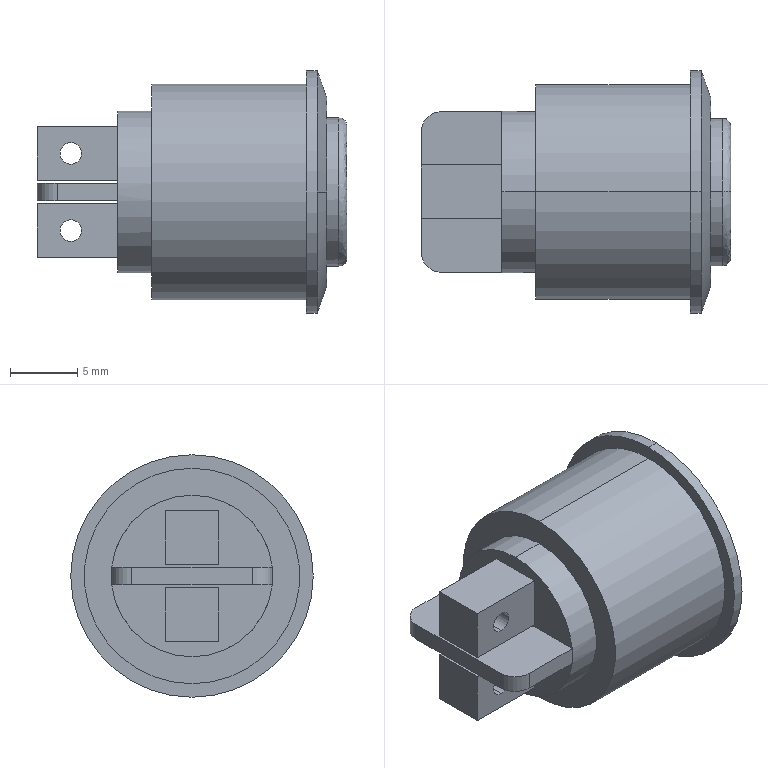Part | SolidWorks | features BaseBody 1 | 1 solid | 41 faces | box 23 x 18 x 18 mm | volume 3351 mm3 | plane 23 | cylinder 14 | spline 2 | cone 2 | commonest cylinder face diameters 1.6 x4 3 x2 11 x2 12 x2 16 x2 18 x2
STEP:
#1=CARTESIAN_POINT('',(3.,0.,4.9));
#2=VERTEX_POINT('',#1);
#3=CARTESIAN_POINT('',(3.,0.04193,4.9));
#4=VERTEX_POINT('',#3);
#5=CARTESIAN_POINT('',(3.,0.,4.9));
#6=CARTESIAN_POINT('',(3.,0.01398,4.9));
#7=CARTESIAN_POINT('',(3.,0.02796,4.9));
#8=CARTESIAN_POINT('',(3.,0.04193,4.9));
#9=(BOUNDED_CURVE()B_SPLINE_CURVE(3,(#5,#6,#7,#8),.UNSPECIFIED.,.F.,.F.)B_SPLINE_CURVE_WITH_KNOTS((4,4),(0.,0.002724),.UNSPECIFIED.)CURVE()GEOMETRIC_REPRESENTATION_ITEM()RATIONAL_B_SPLINE_CURVE((1.,1.,1.,1.))REPRESENTATION_ITEM(''));
#10=EDGE_CURVE('',#2,#4,#9,.T.);
#11=ORIENTED_EDGE('',*,*,#10,.T.);
#12=CARTESIAN_POINT('',(2.4,0.04707,5.5));
#13=VERTEX_POINT('',#12);
#14=CARTESIAN_POINT('',(2.4,0.04193,4.9));
#15=DIRECTION('',(0.,-1.,0.008558));
#16=DIRECTION('',(0.,0.008558,1.));
#17=AXIS2_PLACEMENT_3D('',#14,#15,#16);
#18=CIRCLE('',#17,0.6);
#19=EDGE_CURVE('',#4,#13,#18,.T.);
#20=ORIENTED_EDGE('',*,*,#19,.T.);
#21=CARTESIAN_POINT('',(2.4,0.,5.5));
#22=VERTEX_POINT('',#21);
#23=CARTESIAN_POINT('',(2.4,0.,0.));
#24=DIRECTION('',(-1.,0.,0.));
#25=DIRECTION('',(0.,0.,-1.));
#26=AXIS2_PLACEMENT_3D('',#23,#24,#25);
#27=CIRCLE('',#26,5.5);
#28=EDGE_CURVE('',#22,#13,#27,.T.);
#29=ORIENTED_EDGE('',*,*,#28,.F.);
#30=CARTESIAN_POINT('',(2.4,-0.04707,-5.5));
#31=VERTEX_POINT('',#30);
#32=CARTESIAN_POINT('',(2.4,0.,0.));
#33=DIRECTION('',(-1.,0.,0.));
#34=DIRECTION('',(0.,0.,-1.));
#35=AXIS2_PLACEMENT_3D('',#32,#33,#34);
#36=CIRCLE('',#35,5.5);
#37=EDGE_CURVE('',#31,#22,#36,.T.);
#38=ORIENTED_EDGE('',*,*,#37,.F.);
#39=CARTESIAN_POINT('',(3.,-0.04193,-4.9));
#40=VERTEX_POINT('',#39);
#41=CARTESIAN_POINT('',(2.4,-0.04193,-4.9));
#42=DIRECTION('',(0.,1.,-0.008558));
#43=DIRECTION('',(0.,-0.008558,-1.));
#44=AXIS2_PLACEMENT_3D('',#41,#42,#43);
#45=CIRCLE('',#44,0.6);
#46=EDGE_CURVE('',#40,#31,#45,.T.);
#47=ORIENTED_EDGE('',*,*,#46,.F.);
#48=CARTESIAN_POINT('',(3.,-0.04193,-4.9));
#49=CARTESIAN_POINT('',(3.,-0.1202,-4.899));
#50=CARTESIAN_POINT('',(3.,-0.2018,-4.897));
#51=CARTESIAN_POINT('',(3.,-0.3615,-4.887));
#52=CARTESIAN_POINT('',(3.,-0.4412,-4.881));
#53=CARTESIAN_POINT('',(3.,-0.6798,-4.855));
#54=CARTESIAN_POINT('',(3.,-0.838,-4.831));
#55=CARTESIAN_POINT('',(3.,-1.308,-4.733));
#56=CARTESIAN_POINT('',(3.,-1.615,-4.637));
#57=CARTESIAN_POINT('',(3.,-2.498,-4.264));
#58=CARTESIAN_POINT('',(3.,-3.038,-3.898));
#59=CARTESIAN_POINT('',(3.,-3.937,-2.987));
#60=CARTESIAN_POINT('',(3.,-4.296,-2.443));
#61=CARTESIAN_POINT('',(3.,-4.779,-1.258));
#62=CARTESIAN_POINT('',(3.,-4.903,-0.6179));
#63=CARTESIAN_POINT('',(3.,-4.9,0.02429));
#64=CARTESIAN_POINT('',(3.,-4.9,0.02398));
#65=CARTESIAN_POINT('',(3.,-4.9,0.02623));
#66=CARTESIAN_POINT('',(3.,-4.9,0.02966));
#67=CARTESIAN_POINT('',(3.,-4.9,0.03811));
#68=CARTESIAN_POINT('',(3.,-4.9,0.05674));
#69=CARTESIAN_POINT('',(3.,-4.899,0.07569));
#70=CARTESIAN_POINT('',(3.,-4.899,0.1176));
#71=CARTESIAN_POINT('',(3.,-4.898,0.1508));
#72=CARTESIAN_POINT('',(3.,-4.894,0.2663));
#73=CARTESIAN_POINT('',(3.,-4.888,0.3645));
#74=CARTESIAN_POINT('',(3.,-4.876,0.4909));
#75=CARTESIAN_POINT('',(3.,-4.875,0.4945));
#76=CARTESIAN_POINT('',(3.,-4.874,0.5055));
#77=CARTESIAN_POINT('',(3.,-4.873,0.5219));
#78=CARTESIAN_POINT('',(3.,-4.869,0.5595));
#79=CARTESIAN_POINT('',(3.,-4.86,0.6327));
#80=CARTESIAN_POINT('',(3.,-4.852,0.6918));
#81=CARTESIAN_POINT('',(3.,-4.835,0.8051));
#82=CARTESIAN_POINT('',(3.,-4.823,0.8742));
#83=CARTESIAN_POINT('',(3.,-4.809,0.9447));
#84=CARTESIAN_POINT('',(3.,-4.807,0.9557));
#85=CARTESIAN_POINT('',(3.,-4.803,0.9746));
#86=CARTESIAN_POINT('',(3.,-4.797,1.003));
#87=CARTESIAN_POINT('',(3.,-4.783,1.069));
#88=CARTESIAN_POINT('',(3.,-4.753,1.2));
#89=CARTESIAN_POINT('',(3.,-4.723,1.311));
#90=CARTESIAN_POINT('',(3.,-4.657,1.532));
#91=CARTESIAN_POINT('',(3.,-4.607,1.677));
#92=CARTESIAN_POINT('',(3.,-4.549,1.822));
#93=CARTESIAN_POINT('',(3.,-4.549,1.82));
#94=CARTESIAN_POINT('',(3.,-4.549,1.821));
#95=CARTESIAN_POINT('',(3.,-4.549,1.822));
#96=CARTESIAN_POINT('',(3.,-4.547,1.827));
#97=CARTESIAN_POINT('',(3.,-4.544,1.833));
#98=CARTESIAN_POINT('',(3.,-4.538,1.848));
#99=CARTESIAN_POINT('',(3.,-4.532,1.863));
#100=CARTESIAN_POINT('',(3.,-4.508,1.92));
#101=CARTESIAN_POINT('',(3.,-4.485,1.975));
#102=CARTESIAN_POINT('',(3.,-4.45,2.051));
#103=CARTESIAN_POINT('',(3.,-4.449,2.053));
#104=CARTESIAN_POINT('',(3.,-4.447,2.058));
#105=CARTESIAN_POINT('',(3.,-4.443,2.067));
#106=CARTESIAN_POINT('',(3.,-4.434,2.087));
#107=CARTESIAN_POINT('',(3.,-4.416,2.124));
#108=CARTESIAN_POINT('',(3.,-4.402,2.153));
#109=CARTESIAN_POINT('',(3.,-4.374,2.209));
#110=CARTESIAN_POINT('',(3.,-4.358,2.241));
#111=CARTESIAN_POINT('',(3.,-4.342,2.272));
#112=CARTESIAN_POINT('',(3.,-4.339,2.277));
#113=CARTESIAN_POINT('',(3.,-4.334,2.287));
#114=CARTESIAN_POINT('',(3.,-4.327,2.3));
#115=CARTESIAN_POINT('',(3.,-4.31,2.332));
#116=CARTESIAN_POINT('',(3.,-4.275,2.395));
#117=CARTESIAN_POINT('',(3.,-4.204,2.52));
#118=CARTESIAN_POINT('',(3.,-4.138,2.625));
#119=CARTESIAN_POINT('',(3.,-4.048,2.762));
#120=CARTESIAN_POINT('',(3.,-3.999,2.833));
#121=CARTESIAN_POINT('',(3.,-3.899,2.968));
#122=CARTESIAN_POINT('',(3.,-3.848,3.035));
#123=CARTESIAN_POINT('',(3.,-3.689,3.23));
#124=CARTESIAN_POINT('',(3.,-3.576,3.355));
#125=CARTESIAN_POINT('',(3.,-3.455,3.475));
#126=CARTESIAN_POINT('',(3.,-3.454,3.475));
#127=CARTESIAN_POINT('',(3.,-3.452,3.477));
#128=CARTESIAN_POINT('',(3.,-3.449,3.48));
#129=CARTESIAN_POINT('',(3.,-3.442,3.487));
#130=CARTESIAN_POINT('',(3.,-3.427,3.502));
#131=CARTESIAN_POINT('',(3.,-3.396,3.532));
#132=CARTESIAN_POINT('',(3.,-3.367,3.56));
#133=CARTESIAN_POINT('',(3.,-3.304,3.619));
#134=CARTESIAN_POINT('',(3.,-3.257,3.661));
#135=CARTESIAN_POINT('',(3.,-3.101,3.797));
#136=CARTESIAN_POINT('',(3.,-2.974,3.899));
#137=CARTESIAN_POINT('',(3.,-2.671,4.113));
#138=CARTESIAN_POINT('',(3.,-2.493,4.225));
#139=CARTESIAN_POINT('',(3.,-2.235,4.361));
#140=CARTESIAN_POINT('',(3.,-2.184,4.387));
#141=CARTESIAN_POINT('',(3.,-2.059,4.447));
#142=CARTESIAN_POINT('',(3.,-2.002,4.473));
#143=CARTESIAN_POINT('',(3.,-1.847,4.54));
#144=CARTESIAN_POINT('',(3.,-1.767,4.571));
#145=CARTESIAN_POINT('',(3.,-1.683,4.602));
#146=CARTESIAN_POINT('',(3.,-1.661,4.61));
#147=CARTESIAN_POINT('',(3.,-1.638,4.618));
#148=CARTESIAN_POINT('',(3.,-1.632,4.62));
#149=CARTESIAN_POINT('',(3.,-1.622,4.624));
#150=CARTESIAN_POINT('',(3.,-1.599,4.632));
#151=CARTESIAN_POINT('',(3.,-1.509,4.663));
#152=CARTESIAN_POINT('',(3.,-1.362,4.709));
#153=CARTESIAN_POINT('',(3.,-1.214,4.748));
#154=CARTESIAN_POINT('',(3.,-1.121,4.771));
#155=CARTESIAN_POINT('',(3.,-1.1,4.776));
#156=CARTESIAN_POINT('',(3.,-1.074,4.782));
#157=CARTESIAN_POINT('',(3.,-1.033,4.791));
#158=CARTESIAN_POINT('',(3.,-0.9859,4.801));
#159=CARTESIAN_POINT('',(3.,-0.8851,4.821));
#160=CARTESIAN_POINT('',(3.,-0.808,4.835));
#161=CARTESIAN_POINT('',(3.,-0.6773,4.854));
#162=CARTESIAN_POINT('',(3.,-0.6312,4.86));
#163=CARTESIAN_POINT('',(3.,-0.5705,4.867));
#164=CARTESIAN_POINT('',(3.,-0.5598,4.868));
#165=CARTESIAN_POINT('',(3.,-0.5266,4.872));
#166=CARTESIAN_POINT('',(3.,-0.478,4.877));
#167=CARTESIAN_POINT('',(3.,-0.4326,4.881));
#168=CARTESIAN_POINT('',(3.,-0.1738,4.902));
#169=CARTESIAN_POINT('',(3.,-0.03871,4.9));
#170=CARTESIAN_POINT('',(3.,0.,4.9));
#171=B_SPLINE_CURVE_WITH_KNOTS('',3,(#48,#49,#50,#51,#52,#53,#54,#55,#56,#57,#58,#59,#60,#61,#62,#63,#64,#65,#66,#67,#68,#69,#70,#71,#72,#73,#74,#75,#76,#77,#78,#79,#80,#81,#82,#83,#84,#85,#86,#87,#88,#89,#90,#91,#92,#93,#94,#95,#96,#97,#98,#99,#100,#101,#102,#103,#104,#105,#106,#107,#108,#109,#110,#111,#112,#113,#114,#115,#116,#117,#118,#119,#120,#121,#122,#123,#124,#125,#126,#127,#128,#129,#130,#131,#132,#133,#134,#135,#136,#137,#138,#139,#140,#141,#142,#143,#144,#145,#146,#147,#148,#149,#150,#151,#152,#153,#154,#155,#156,#157,#158,#159,#160,#161,#162,#163,#164,#165,#166,#167,#168,#169,#170),.UNSPECIFIED.,.F.,.F.,(4,2,2,2,2,2,2,2,2,1,1,1,2,2,2,2,1,1,1,2,2,2,1,1,1,2,2,2,1,1,2,2,2,2,1,1,1,2,2,2,1,1,1,1,2,2,2,2,2,1,1,1,1,2,2,2,2,2,2,2,2,2,2,1,2,2,1,2,2,2,2,1,2,4),(0.002914,0.01849,0.03407,0.06523,0.1276,0.2522,0.3768,0.5015,0.5019,0.5024,0.5034,0.5054,0.5092,0.517,0.5326,0.5336,0.5346,0.5365,0.5404,0.5482,0.5638,0.5657,0.5677,0.5716,0.5794,0.5949,0.6261,0.6266,0.6271,0.628,0.63,0.6339,0.6417,0.6422,0.6426,0.6436,0.6456,0.6495,0.6573,0.6582,0.6592,0.6611,0.665,0.6728,0.6884,0.704,0.7196,0.7507,0.7512,0.7517,0.7527,0.7546,0.7585,0.7663,0.7819,0.813,0.8442,0.852,0.8598,0.8754,0.8832,0.887,0.8909,0.9065,0.9221,0.926,0.9299,0.9377,0.9533,0.9611,0.963,0.9649,0.9688,1.),.UNSPECIFIED.);
#172=EDGE_CURVE('',#40,#2,#171,.T.);
#173=ORIENTED_EDGE('',*,*,#172,.T.);
#174=EDGE_LOOP('',(#11,#20,#29,#38,#47,#173));
#175=FACE_OUTER_BOUND('',#174,.T.);
#176=CARTESIAN_POINT('',(3.,0.04188,4.894));
#177=CARTESIAN_POINT('',(3.,-2.825,4.919));
#178=CARTESIAN_POINT('',(3.,-4.869,2.909));
#179=CARTESIAN_POINT('',(3.,-4.894,0.04188));
#180=CARTESIAN_POINT('',(3.,-4.919,-2.825));
#181=CARTESIAN_POINT('',(3.,-2.909,-4.869));
#182=CARTESIAN_POINT('',(3.,-0.04188,-4.894));
#183=CARTESIAN_POINT('',(3.003,0.04491,5.248));
#184=CARTESIAN_POINT('',(3.003,-3.029,5.274));
#185=CARTESIAN_POINT('',(3.003,-5.222,3.119));
#186=CARTESIAN_POINT('',(3.003,-5.248,0.04491));
#187=CARTESIAN_POINT('',(3.003,-5.274,-3.029));
#188=CARTESIAN_POINT('',(3.003,-3.119,-5.222));
#189=CARTESIAN_POINT('',(3.003,-0.04491,-5.248));
#190=CARTESIAN_POINT('',(2.754,0.04707,5.5));
#191=CARTESIAN_POINT('',(2.754,-3.175,5.527));
#192=CARTESIAN_POINT('',(2.754,-5.472,3.269));
#193=CARTESIAN_POINT('',(2.754,-5.5,0.04707));
#194=CARTESIAN_POINT('',(2.754,-5.527,-3.175));
#195=CARTESIAN_POINT('',(2.754,-3.269,-5.472));
#196=CARTESIAN_POINT('',(2.754,-0.04707,-5.5));
#197=CARTESIAN_POINT('',(2.4,0.04707,5.5));
#198=CARTESIAN_POINT('',(2.4,-3.175,5.527));
#199=CARTESIAN_POINT('',(2.4,-5.472,3.269));
#200=CARTESIAN_POINT('',(2.4,-5.5,0.04707));
#201=CARTESIAN_POINT('',(2.4,-5.527,-3.175));
#202=CARTESIAN_POINT('',(2.4,-3.269,-5.472));
#203=CARTESIAN_POINT('',(2.4,-0.04707,-5.5));
#204=(BOUNDED_SURFACE()B_SPLINE_SURFACE(3,3,((#176,#177,#178,#179,#180,#181,#182),(#183,#184,#185,#186,#187,#188,#189),(#190,#191,#192,#193,#194,#195,#196),(#197,#198,#199,#200,#201,#202,#203)),.UNSPECIFIED.,.F.,.F.,.F.)B_SPLINE_SURFACE_WITH_KNOTS((4,4),(4,3,4),(0.,1.),(0.,0.5,1.),.UNSPECIFIED.)GEOMETRIC_REPRESENTATION_ITEM()RATIONAL_B_SPLINE_SURFACE(((1.,0.8047,0.8047,1.,0.8047,0.8047,1.),(0.8024,0.6458,0.6458,0.8024,0.6458,0.6458,0.8024),(0.8024,0.6458,0.6458,0.8024,0.6458,0.6458,0.8024),(1.,0.8047,0.8047,1.,0.8047,0.8047,1.)))REPRESENTATION_ITEM('')SURFACE());
#205=ADVANCED_FACE('',(#175),#204,.T.);
#206=CARTESIAN_POINT('',(0.,0.,8.));
#207=VERTEX_POINT('',#206);
#208=CARTESIAN_POINT('',(0.,0.,-8.));
#209=VERTEX_POINT('',#208);
#210=CARTESIAN_POINT('',(0.,0.,0.));
#211=DIRECTION('',(-1.,0.,0.));
#212=DIRECTION('',(0.,0.,1.));
#213=AXIS2_PLACEMENT_3D('',#210,#211,#212);
#214=CIRCLE('',#213,8.);
#215=EDGE_CURVE('',#207,#209,#214,.T.);
#216=ORIENTED_EDGE('',*,*,#215,.T.);
#217=CARTESIAN_POINT('',(-11.5,0.,-8.));
#218=VERTEX_POINT('',#217);
#219=CARTESIAN_POINT('',(2.275,0.,-8.));
#220=DIRECTION('',(-1.,0.,0.));
#221=VECTOR('',#220,1000.);
#222=LINE('',#219,#221);
#223=EDGE_CURVE('',#209,#218,#222,.T.);
#224=ORIENTED_EDGE('',*,*,#223,.T.);
#225=CARTESIAN_POINT('',(-11.5,0.,8.));
#226=VERTEX_POINT('',#225);
#227=CARTESIAN_POINT('',(-11.5,0.,0.));
#228=DIRECTION('',(1.,0.,0.));
#229=DIRECTION('',(0.,0.,1.));
#230=AXIS2_PLACEMENT_3D('',#227,#228,#229);
#231=CIRCLE('',#230,8.);
#232=EDGE_CURVE('',#218,#226,#231,.T.);
#233=ORIENTED_EDGE('',*,*,#232,.T.);
#234=CARTESIAN_POINT('',(2.275,0.,8.));
#235=DIRECTION('',(-1.,0.,0.));
#236=VECTOR('',#235,1000.);
#237=LINE('',#234,#236);
#238=EDGE_CURVE('',#207,#226,#237,.T.);
#239=ORIENTED_EDGE('',*,*,#238,.F.);
#240=EDGE_LOOP('',(#216,#224,#233,#239));
#241=FACE_OUTER_BOUND('',#240,.T.);
#242=CARTESIAN_POINT('',(2.275,0.,0.));
#243=DIRECTION('',(-1.,0.,0.));
#244=DIRECTION('',(0.,0.,1.));
#245=AXIS2_PLACEMENT_3D('',#242,#243,#244);
#246=CYLINDRICAL_SURFACE('',#245,8.);
#247=ADVANCED_FACE('',(#241),#246,.T.);
#248=CARTESIAN_POINT('',(-11.5,0.,-6.));
#249=VERTEX_POINT('',#248);
#250=CARTESIAN_POINT('',(-11.5,0.,6.));
#251=VERTEX_POINT('',#250);
#252=CARTESIAN_POINT('',(-11.5,0.,0.));
#253=DIRECTION('',(1.,0.,0.));
#254=DIRECTION('',(0.,0.,1.));
#255=AXIS2_PLACEMENT_3D('',#252,#253,#254);
#256=CIRCLE('',#255,6.);
#257=EDGE_CURVE('',#249,#251,#256,.T.);
#258=ORIENTED_EDGE('',*,*,#257,.F.);
#259=CARTESIAN_POINT('',(-14.,0.,-6.));
#260=VERTEX_POINT('',#259);
#261=CARTESIAN_POINT('',(-14.,0.,-6.));
#262=DIRECTION('',(-1.,0.,0.));
#263=VECTOR('',#262,1000.);
#264=LINE('',#261,#263);
#265=EDGE_CURVE('',#249,#260,#264,.T.);
#266=ORIENTED_EDGE('',*,*,#265,.T.);
#267=CARTESIAN_POINT('',(-14.,5.963,-0.6628));
#268=VERTEX_POINT('',#267);
#269=CARTESIAN_POINT('',(-14.,0.,0.));
#270=DIRECTION('',(1.,0.,0.));
#271=DIRECTION('',(0.,0.,1.));
#272=AXIS2_PLACEMENT_3D('',#269,#270,#271);
#273=CIRCLE('',#272,6.);
#274=EDGE_CURVE('',#260,#268,#273,.T.);
#275=ORIENTED_EDGE('',*,*,#274,.T.);
#276=CARTESIAN_POINT('',(-14.,5.963,0.6628));
#277=VERTEX_POINT('',#276);
#278=CARTESIAN_POINT('',(-14.,0.,0.));
#279=DIRECTION('',(1.,0.,0.));
#280=DIRECTION('',(0.,0.,1.));
#281=AXIS2_PLACEMENT_3D('',#278,#279,#280);
#282=CIRCLE('',#281,6.);
#283=EDGE_CURVE('',#268,#277,#282,.T.);
#284=ORIENTED_EDGE('',*,*,#283,.T.);
#285=CARTESIAN_POINT('',(-14.,0.,6.));
#286=VERTEX_POINT('',#285);
#287=CARTESIAN_POINT('',(-14.,0.,0.));
#288=DIRECTION('',(1.,0.,0.));
#289=DIRECTION('',(0.,0.,1.));
#290=AXIS2_PLACEMENT_3D('',#287,#288,#289);
#291=CIRCLE('',#290,6.);
#292=EDGE_CURVE('',#277,#286,#291,.T.);
#293=ORIENTED_EDGE('',*,*,#292,.T.);
#294=CARTESIAN_POINT('',(-14.,0.,6.));
#295=DIRECTION('',(-1.,0.,0.));
#296=VECTOR('',#295,1000.);
#297=LINE('',#294,#296);
#298=EDGE_CURVE('',#251,#286,#297,.T.);
#299=ORIENTED_EDGE('',*,*,#298,.F.);
#300=EDGE_LOOP('',(#258,#266,#275,#284,#293,#299));
#301=FACE_OUTER_BOUND('',#300,.T.);
#302=CARTESIAN_POINT('',(-14.,0.,0.));
#303=DIRECTION('',(-1.,0.,0.));
#304=DIRECTION('',(0.,0.,1.));
#305=AXIS2_PLACEMENT_3D('',#302,#303,#304);
#306=CYLINDRICAL_SURFACE('',#305,6.);
#307=ADVANCED_FACE('',(#301),#306,.T.);
#308=CARTESIAN_POINT('',(0.8,9.,0.));
#309=VERTEX_POINT('',#308);
#310=CARTESIAN_POINT('',(0.8,0.,-9.));
#311=VERTEX_POINT('',#310);
#312=CARTESIAN_POINT('',(0.8,0.,0.));
#313=DIRECTION('',(-1.,0.,0.));
#314=DIRECTION('',(0.,0.,1.));
#315=AXIS2_PLACEMENT_3D('',#312,#313,#314);
#316=CIRCLE('',#315,9.);
#317=EDGE_CURVE('',#309,#311,#316,.T.);
#318=ORIENTED_EDGE('',*,*,#317,.T.);
#319=CARTESIAN_POINT('',(0.,0.,-9.));
#320=VERTEX_POINT('',#319);
#321=CARTESIAN_POINT('',(2.275,0.,-9.));
#322=DIRECTION('',(-1.,0.,0.));
#323=VECTOR('',#322,1000.);
#324=LINE('',#321,#323);
#325=EDGE_CURVE('',#311,#320,#324,.T.);
#326=ORIENTED_EDGE('',*,*,#325,.T.);
#327=CARTESIAN_POINT('',(0.,0.,9.));
#328=VERTEX_POINT('',#327);
#329=CARTESIAN_POINT('',(0.,0.,0.));
#330=DIRECTION('',(-1.,0.,0.));
#331=DIRECTION('',(0.,0.,1.));
#332=AXIS2_PLACEMENT_3D('',#329,#330,#331);
#333=CIRCLE('',#332,9.);
#334=EDGE_CURVE('',#328,#320,#333,.T.);
#335=ORIENTED_EDGE('',*,*,#334,.F.);
#336=CARTESIAN_POINT('',(0.8,0.,9.));
#337=VERTEX_POINT('',#336);
#338=CARTESIAN_POINT('',(2.275,0.,9.));
#339=DIRECTION('',(-1.,0.,0.));
#340=VECTOR('',#339,1000.);
#341=LINE('',#338,#340);
#342=EDGE_CURVE('',#337,#328,#341,.T.);
#343=ORIENTED_EDGE('',*,*,#342,.F.);
#344=CARTESIAN_POINT('',(0.8,0.,0.));
#345=DIRECTION('',(-1.,0.,0.));
#346=DIRECTION('',(0.,0.,1.));
#347=AXIS2_PLACEMENT_3D('',#344,#345,#346);
#348=CIRCLE('',#347,9.);
#349=EDGE_CURVE('',#337,#309,#348,.T.);
#350=ORIENTED_EDGE('',*,*,#349,.T.);
#351=EDGE_LOOP('',(#318,#326,#335,#343,#350));
#352=FACE_OUTER_BOUND('',#351,.T.);
#353=CARTESIAN_POINT('',(2.275,0.,0.));
#354=DIRECTION('',(-1.,0.,0.));
#355=DIRECTION('',(0.,0.,1.));
#356=AXIS2_PLACEMENT_3D('',#353,#354,#355);
#357=CYLINDRICAL_SURFACE('',#356,9.);
#358=ADVANCED_FACE('',(#352),#357,.T.);
#359=CARTESIAN_POINT('',(1.5,-7.,0.));
#360=VERTEX_POINT('',#359);
#361=CARTESIAN_POINT('',(1.5,7.,0.));
#362=VERTEX_POINT('',#361);
#363=CARTESIAN_POINT('',(1.5,0.,0.));
#364=DIRECTION('',(-1.,0.,0.));
#365=DIRECTION('',(0.,-1.,0.));
#366=AXIS2_PLACEMENT_3D('',#363,#364,#365);
#367=CIRCLE('',#366,7.);
#368=EDGE_CURVE('',#360,#362,#367,.T.);
#369=ORIENTED_EDGE('',*,*,#368,.T.);
#370=CARTESIAN_POINT('',(0.8,9.,0.));
#371=DIRECTION('',(-0.3304,0.9439,0.));
#372=VECTOR('',#371,1000.);
#373=LINE('',#370,#372);
#374=EDGE_CURVE('',#362,#309,#373,.T.);
#375=ORIENTED_EDGE('',*,*,#374,.T.);
#376=ORIENTED_EDGE('',*,*,#349,.F.);
#377=CARTESIAN_POINT('',(0.8,-9.,0.));
#378=VERTEX_POINT('',#377);
#379=CARTESIAN_POINT('',(0.8,0.,0.));
#380=DIRECTION('',(-1.,0.,0.));
#381=DIRECTION('',(0.,0.,1.));
#382=AXIS2_PLACEMENT_3D('',#379,#380,#381);
#383=CIRCLE('',#382,9.);
#384=EDGE_CURVE('',#378,#337,#383,.T.);
#385=ORIENTED_EDGE('',*,*,#384,.F.);
#386=CARTESIAN_POINT('',(0.8,-9.,0.));
#387=DIRECTION('',(-0.3304,-0.9439,0.));
#388=VECTOR('',#387,1000.);
#389=LINE('',#386,#388);
#390=EDGE_CURVE('',#360,#378,#389,.T.);
#391=ORIENTED_EDGE('',*,*,#390,.F.);
#392=EDGE_LOOP('',(#369,#375,#376,#385,#391));
#393=FACE_OUTER_BOUND('',#392,.T.);
#394=CARTESIAN_POINT('',(0.8,0.,0.));
#395=DIRECTION('',(-1.,0.,0.));
#396=DIRECTION('',(0.,-1.,0.));
#397=AXIS2_PLACEMENT_3D('',#394,#395,#396);
#398=CONICAL_SURFACE('',#397,9.,1.234);
#399=ADVANCED_FACE('',(#393),#398,.T.);
#400=CARTESIAN_POINT('',(-17.495,-2.,-2.063));
#401=VERTEX_POINT('',#400);
#402=CARTESIAN_POINT('',(-17.495,-2.,-3.663));
#403=VERTEX_POINT('',#402);
#404=CARTESIAN_POINT('',(-17.495,-2.,-2.863));
#405=DIRECTION('',(0.,-1.,0.));
#406=DIRECTION('',(0.,0.,1.));
#407=AXIS2_PLACEMENT_3D('',#404,#405,#406);
#408=CIRCLE('',#407,0.8);
#409=EDGE_CURVE('',#401,#403,#408,.T.);
#410=ORIENTED_EDGE('',*,*,#409,.T.);
#411=CARTESIAN_POINT('',(-17.495,2.,-3.663));
#412=VERTEX_POINT('',#411);
#413=CARTESIAN_POINT('',(-17.495,-2.,-3.663));
#414=DIRECTION('',(0.,1.,0.));
#415=VECTOR('',#414,1000.);
#416=LINE('',#413,#415);
#417=EDGE_CURVE('',#403,#412,#416,.T.);
#418=ORIENTED_EDGE('',*,*,#417,.T.);
#419=CARTESIAN_POINT('',(-17.495,2.,-2.063));
#420=VERTEX_POINT('',#419);
#421=CARTESIAN_POINT('',(-17.495,2.,-2.863));
#422=DIRECTION('',(0.,1.,0.));
#423=DIRECTION('',(0.,0.,1.));
#424=AXIS2_PLACEMENT_3D('',#421,#422,#423);
#425=CIRCLE('',#424,0.8);
#426=EDGE_CURVE('',#412,#420,#425,.T.);
#427=ORIENTED_EDGE('',*,*,#426,.T.);
#428=CARTESIAN_POINT('',(-17.495,-2.,-2.063));
#429=DIRECTION('',(0.,1.,0.));
#430=VECTOR('',#429,1000.);
#431=LINE('',#428,#430);
#432=EDGE_CURVE('',#401,#420,#431,.T.);
#433=ORIENTED_EDGE('',*,*,#432,.F.);
#434=EDGE_LOOP('',(#410,#418,#427,#433));
#435=FACE_OUTER_BOUND('',#434,.T.);
#436=CARTESIAN_POINT('',(-17.495,-2.,-2.863));
#437=DIRECTION('',(0.,1.,0.));
#438=DIRECTION('',(0.,0.,1.));
#439=AXIS2_PLACEMENT_3D('',#436,#437,#438);
#440=CYLINDRICAL_SURFACE('',#439,0.8);
#441=ADVANCED_FACE('',(#435),#440,.F.);
#442=CARTESIAN_POINT('',(-17.495,2.,3.663));
#443=VERTEX_POINT('',#442);
#444=CARTESIAN_POINT('',(-17.495,2.,2.063));
#445=VERTEX_POINT('',#444);
#446=CARTESIAN_POINT('',(-17.495,2.,2.863));
#447=DIRECTION('',(0.,-1.,0.));
#448=DIRECTION('',(0.,0.,-1.));
#449=AXIS2_PLACEMENT_3D('',#446,#447,#448);
#450=CIRCLE('',#449,0.8);
#451=EDGE_CURVE('',#443,#445,#450,.T.);
#452=ORIENTED_EDGE('',*,*,#451,.F.);
#453=CARTESIAN_POINT('',(-17.495,-2.,3.663));
#454=VERTEX_POINT('',#453);
#455=CARTESIAN_POINT('',(-17.495,-2.,3.663));
#456=DIRECTION('',(0.,-1.,0.));
#457=VECTOR('',#456,1000.);
#458=LINE('',#455,#457);
#459=EDGE_CURVE('',#443,#454,#458,.T.);
#460=ORIENTED_EDGE('',*,*,#459,.T.);
#461=CARTESIAN_POINT('',(-17.495,-2.,2.063));
#462=VERTEX_POINT('',#461);
#463=CARTESIAN_POINT('',(-17.495,-2.,2.863));
#464=DIRECTION('',(0.,1.,0.));
#465=DIRECTION('',(0.,0.,-1.));
#466=AXIS2_PLACEMENT_3D('',#463,#464,#465);
#467=CIRCLE('',#466,0.8);
#468=EDGE_CURVE('',#462,#454,#467,.T.);
#469=ORIENTED_EDGE('',*,*,#468,.F.);
#470=CARTESIAN_POINT('',(-17.495,-2.,2.063));
#471=DIRECTION('',(0.,-1.,0.));
#472=VECTOR('',#471,1000.);
#473=LINE('',#470,#472);
#474=EDGE_CURVE('',#445,#462,#473,.T.);
#475=ORIENTED_EDGE('',*,*,#474,.F.);
#476=EDGE_LOOP('',(#452,#460,#469,#475));
#477=FACE_OUTER_BOUND('',#476,.T.);
#478=CARTESIAN_POINT('',(-17.495,-2.,2.863));
#479=DIRECTION('',(0.,-1.,0.));
#480=DIRECTION('',(0.,0.,-1.));
#481=AXIS2_PLACEMENT_3D('',#478,#479,#480);
#482=CYLINDRICAL_SURFACE('',#481,0.8);
#483=ADVANCED_FACE('',(#477),#482,.F.);
#484=CARTESIAN_POINT('',(1.5,0.,-5.5));
#485=VERTEX_POINT('',#484);
#486=CARTESIAN_POINT('',(1.5,0.,5.5));
#487=VERTEX_POINT('',#486);
#488=CARTESIAN_POINT('',(1.5,0.,0.));
#489=DIRECTION('',(1.,0.,0.));
#490=DIRECTION('',(0.,0.,-1.));
#491=AXIS2_PLACEMENT_3D('',#488,#489,#490);
#492=CIRCLE('',#491,5.5);
#493=EDGE_CURVE('',#485,#487,#492,.T.);
#494=ORIENTED_EDGE('',*,*,#493,.T.);
#495=CARTESIAN_POINT('',(1.5,0.,5.5));
#496=DIRECTION('',(1.,0.,0.));
#497=VECTOR('',#496,1000.);
#498=LINE('',#495,#497);
#499=EDGE_CURVE('',#487,#22,#498,.T.);
#500=ORIENTED_EDGE('',*,*,#499,.T.);
#501=ORIENTED_EDGE('',*,*,#28,.T.);
#502=CARTESIAN_POINT('',(2.4,0.,-5.5));
#503=VERTEX_POINT('',#502);
#504=CARTESIAN_POINT('',(2.4,0.,0.));
#505=DIRECTION('',(-1.,0.,0.));
#506=DIRECTION('',(0.,0.,-1.));
#507=AXIS2_PLACEMENT_3D('',#504,#505,#506);
#508=CIRCLE('',#507,5.5);
#509=EDGE_CURVE('',#13,#503,#508,.T.);
#510=ORIENTED_EDGE('',*,*,#509,.T.);
#511=CARTESIAN_POINT('',(1.5,0.,-5.5));
#512=DIRECTION('',(1.,0.,0.));
#513=VECTOR('',#512,1000.);
#514=LINE('',#511,#513);
#515=EDGE_CURVE('',#485,#503,#514,.T.);
#516=ORIENTED_EDGE('',*,*,#515,.F.);
#517=EDGE_LOOP('',(#494,#500,#501,#510,#516));
#518=FACE_OUTER_BOUND('',#517,.T.);
#519=CARTESIAN_POINT('',(1.5,0.,0.));
#520=DIRECTION('',(1.,0.,0.));
#521=DIRECTION('',(0.,0.,-1.));
#522=AXIS2_PLACEMENT_3D('',#519,#520,#521);
#523=CYLINDRICAL_SURFACE('',#522,5.5);
#524=ADVANCED_FACE('',(#518),#523,.T.);
#525=ORIENTED_EDGE('',*,*,#223,.F.);
#526=CARTESIAN_POINT('',(0.,0.,0.));
#527=DIRECTION('',(-1.,0.,0.));
#528=DIRECTION('',(0.,0.,1.));
#529=AXIS2_PLACEMENT_3D('',#526,#527,#528);
#530=CIRCLE('',#529,8.);
#531=EDGE_CURVE('',#209,#207,#530,.T.);
#532=ORIENTED_EDGE('',*,*,#531,.T.);
#533=ORIENTED_EDGE('',*,*,#238,.T.);
#534=CARTESIAN_POINT('',(-11.5,0.,0.));
#535=DIRECTION('',(1.,0.,0.));
#536=DIRECTION('',(0.,0.,1.));
#537=AXIS2_PLACEMENT_3D('',#534,#535,#536);
#538=CIRCLE('',#537,8.);
#539=EDGE_CURVE('',#226,#218,#538,.T.);
#540=ORIENTED_EDGE('',*,*,#539,.T.);
#541=EDGE_LOOP('',(#525,#532,#533,#540));
#542=FACE_OUTER_BOUND('',#541,.T.);
#543=CARTESIAN_POINT('',(2.275,0.,0.));
#544=DIRECTION('',(-1.,0.,0.));
#545=DIRECTION('',(0.,0.,1.));
#546=AXIS2_PLACEMENT_3D('',#543,#544,#545);
#547=CYLINDRICAL_SURFACE('',#546,8.);
#548=ADVANCED_FACE('',(#542),#547,.T.);
#549=CARTESIAN_POINT('',(-11.5,0.,0.));
#550=DIRECTION('',(1.,0.,0.));
#551=DIRECTION('',(0.,0.,1.));
#552=AXIS2_PLACEMENT_3D('',#549,#550,#551);
#553=CIRCLE('',#552,6.);
#554=EDGE_CURVE('',#251,#249,#553,.T.);
#555=ORIENTED_EDGE('',*,*,#554,.T.);
#556=ORIENTED_EDGE('',*,*,#257,.T.);
#557=EDGE_LOOP('',(#555,#556));
#558=FACE_BOUND('',#557,.T.);
#559=ORIENTED_EDGE('',*,*,#539,.F.);
#560=ORIENTED_EDGE('',*,*,#232,.F.);
#561=EDGE_LOOP('',(#559,#560));
#562=FACE_OUTER_BOUND('',#561,.T.);
#563=CARTESIAN_POINT('',(-11.5,0.,0.));
#564=DIRECTION('',(-1.,0.,0.));
#565=DIRECTION('',(0.,0.,1.));
#566=AXIS2_PLACEMENT_3D('',#563,#564,#565);
#567=PLANE('',#566);
#568=ADVANCED_FACE('',(#558,#562),#567,.T.);
#569=ORIENTED_EDGE('',*,*,#215,.F.);
#570=ORIENTED_EDGE('',*,*,#531,.F.);
#571=EDGE_LOOP('',(#569,#570));
#572=FACE_BOUND('',#571,.T.);
#573=ORIENTED_EDGE('',*,*,#334,.T.);
#574=CARTESIAN_POINT('',(0.,0.,0.));
#575=DIRECTION('',(-1.,0.,0.));
#576=DIRECTION('',(0.,0.,1.));
#577=AXIS2_PLACEMENT_3D('',#574,#575,#576);
#578=CIRCLE('',#577,9.);
#579=EDGE_CURVE('',#320,#328,#578,.T.);
#580=ORIENTED_EDGE('',*,*,#579,.T.);
#581=EDGE_LOOP('',(#573,#580));
#582=FACE_OUTER_BOUND('',#581,.T.);
#583=CARTESIAN_POINT('',(0.,0.,0.));
#584=DIRECTION('',(-1.,0.,0.));
#585=DIRECTION('',(0.,0.,1.));
#586=AXIS2_PLACEMENT_3D('',#583,#584,#585);
#587=PLANE('',#586);
#588=ADVANCED_FACE('',(#572,#582),#587,.T.);
#589=ORIENTED_EDGE('',*,*,#265,.F.);
#590=ORIENTED_EDGE('',*,*,#554,.F.);
#591=ORIENTED_EDGE('',*,*,#298,.T.);
#592=CARTESIAN_POINT('',(-14.,-5.963,0.6628));
#593=VERTEX_POINT('',#592);
#594=CARTESIAN_POINT('',(-14.,0.,0.));
#595=DIRECTION('',(1.,0.,0.));
#596=DIRECTION('',(0.,0.,1.));
#597=AXIS2_PLACEMENT_3D('',#594,#595,#596);
#598=CIRCLE('',#597,6.);
#599=EDGE_CURVE('',#286,#593,#598,.T.);
#600=ORIENTED_EDGE('',*,*,#599,.T.);
#601=CARTESIAN_POINT('',(-14.,-5.963,-0.6628));
#602=VERTEX_POINT('',#601);
#603=CARTESIAN_POINT('',(-14.,0.,0.));
#604=DIRECTION('',(1.,0.,0.));
#605=DIRECTION('',(0.,0.,1.));
#606=AXIS2_PLACEMENT_3D('',#603,#604,#605);
#607=CIRCLE('',#606,6.);
#608=EDGE_CURVE('',#593,#602,#607,.T.);
#609=ORIENTED_EDGE('',*,*,#608,.T.);
#610=CARTESIAN_POINT('',(-14.,0.,0.));
#611=DIRECTION('',(1.,0.,0.));
#612=DIRECTION('',(0.,0.,1.));
#613=AXIS2_PLACEMENT_3D('',#610,#611,#612);
#614=CIRCLE('',#613,6.);
#615=EDGE_CURVE('',#602,#260,#614,.T.);
#616=ORIENTED_EDGE('',*,*,#615,.T.);
#617=EDGE_LOOP('',(#589,#590,#591,#600,#609,#616));
#618=FACE_OUTER_BOUND('',#617,.T.);
#619=CARTESIAN_POINT('',(-14.,0.,0.));
#620=DIRECTION('',(-1.,0.,0.));
#621=DIRECTION('',(0.,0.,1.));
#622=AXIS2_PLACEMENT_3D('',#619,#620,#621);
#623=CYLINDRICAL_SURFACE('',#622,6.);
#624=ADVANCED_FACE('',(#618),#623,.T.);
#625=ORIENTED_EDGE('',*,*,#325,.F.);
#626=CARTESIAN_POINT('',(0.8,0.,0.));
#627=DIRECTION('',(-1.,0.,0.));
#628=DIRECTION('',(0.,0.,1.));
#629=AXIS2_PLACEMENT_3D('',#626,#627,#628);
#630=CIRCLE('',#629,9.);
#631=EDGE_CURVE('',#311,#378,#630,.T.);
#632=ORIENTED_EDGE('',*,*,#631,.T.);
#633=ORIENTED_EDGE('',*,*,#384,.T.);
#634=ORIENTED_EDGE('',*,*,#342,.T.);
#635=ORIENTED_EDGE('',*,*,#579,.F.);
#636=EDGE_LOOP('',(#625,#632,#633,#634,#635));
#637=FACE_OUTER_BOUND('',#636,.T.);
#638=CARTESIAN_POINT('',(2.275,0.,0.));
#639=DIRECTION('',(-1.,0.,0.));
#640=DIRECTION('',(0.,0.,1.));
#641=AXIS2_PLACEMENT_3D('',#638,#639,#640);
#642=CYLINDRICAL_SURFACE('',#641,9.);
#643=ADVANCED_FACE('',(#637),#642,.T.);
#644=ORIENTED_EDGE('',*,*,#283,.F.);
#645=CARTESIAN_POINT('',(-14.,5.963,0.6628));
#646=DIRECTION('',(0.,0.,-1.));
#647=VECTOR('',#646,1000.);
#648=LINE('',#645,#647);
#649=EDGE_CURVE('',#277,#268,#648,.T.);
#650=ORIENTED_EDGE('',*,*,#649,.F.);
#651=EDGE_LOOP('',(#644,#650));
#652=FACE_OUTER_BOUND('',#651,.T.);
#653=CARTESIAN_POINT('',(-14.,0.,0.));
#654=DIRECTION('',(-1.,0.,0.));
#655=DIRECTION('',(0.,0.,1.));
#656=AXIS2_PLACEMENT_3D('',#653,#654,#655);
#657=PLANE('',#656);
#658=ADVANCED_FACE('',(#652),#657,.T.);
#659=CARTESIAN_POINT('',(-14.,-2.,-4.863));
#660=VERTEX_POINT('',#659);
#661=CARTESIAN_POINT('',(-14.,2.,-4.863));
#662=VERTEX_POINT('',#661);
#663=CARTESIAN_POINT('',(-14.,0.,-4.863));
#664=DIRECTION('',(0.,1.,0.));
#665=VECTOR('',#664,1000.);
#666=LINE('',#663,#665);
#667=EDGE_CURVE('',#660,#662,#666,.T.);
#668=ORIENTED_EDGE('',*,*,#667,.T.);
#669=CARTESIAN_POINT('',(-14.,2.,-0.8628));
#670=VERTEX_POINT('',#669);
#671=CARTESIAN_POINT('',(-14.,2.,0.));
#672=DIRECTION('',(0.,0.,1.));
#673=VECTOR('',#672,1000.);
#674=LINE('',#671,#673);
#675=EDGE_CURVE('',#662,#670,#674,.T.);
#676=ORIENTED_EDGE('',*,*,#675,.T.);
#677=CARTESIAN_POINT('',(-14.,-2.,-0.8628));
#678=VERTEX_POINT('',#677);
#679=CARTESIAN_POINT('',(-14.,0.,-0.8628));
#680=DIRECTION('',(0.,-1.,0.));
#681=VECTOR('',#680,1000.);
#682=LINE('',#679,#681);
#683=EDGE_CURVE('',#670,#678,#682,.T.);
#684=ORIENTED_EDGE('',*,*,#683,.T.);
#685=CARTESIAN_POINT('',(-14.,-2.,0.));
#686=DIRECTION('',(0.,0.,-1.));
#687=VECTOR('',#686,1000.);
#688=LINE('',#685,#687);
#689=EDGE_CURVE('',#678,#660,#688,.T.);
#690=ORIENTED_EDGE('',*,*,#689,.T.);
#691=EDGE_LOOP('',(#668,#676,#684,#690));
#692=FACE_BOUND('',#691,.T.);
#693=ORIENTED_EDGE('',*,*,#615,.F.);
#694=CARTESIAN_POINT('',(-14.,0.,-0.6628));
#695=DIRECTION('',(0.,1.,0.));
#696=VECTOR('',#695,1000.);
#697=LINE('',#694,#696);
#698=EDGE_CURVE('',#602,#268,#697,.T.);
#699=ORIENTED_EDGE('',*,*,#698,.T.);
#700=ORIENTED_EDGE('',*,*,#274,.F.);
#701=EDGE_LOOP('',(#693,#699,#700));
#702=FACE_OUTER_BOUND('',#701,.T.);
#703=CARTESIAN_POINT('',(-14.,0.,0.));
#704=DIRECTION('',(-1.,0.,0.));
#705=DIRECTION('',(0.,0.,1.));
#706=AXIS2_PLACEMENT_3D('',#703,#704,#705);
#707=PLANE('',#706);
#708=ADVANCED_FACE('',(#692,#702),#707,.T.);
#709=ORIENTED_EDGE('',*,*,#608,.F.);
#710=CARTESIAN_POINT('',(-14.,-5.963,-0.6628));
#711=DIRECTION('',(0.,0.,1.));
#712=VECTOR('',#711,1000.);
#713=LINE('',#710,#712);
#714=EDGE_CURVE('',#602,#593,#713,.T.);
#715=ORIENTED_EDGE('',*,*,#714,.F.);
#716=EDGE_LOOP('',(#709,#715));
#717=FACE_OUTER_BOUND('',#716,.T.);
#718=CARTESIAN_POINT('',(-14.,0.,0.));
#719=DIRECTION('',(-1.,0.,0.));
#720=DIRECTION('',(0.,0.,1.));
#721=AXIS2_PLACEMENT_3D('',#718,#719,#720);
#722=PLANE('',#721);
#723=ADVANCED_FACE('',(#717),#722,.T.);
#724=CARTESIAN_POINT('',(-14.,-2.,0.8628));
#725=VERTEX_POINT('',#724);
#726=CARTESIAN_POINT('',(-14.,2.,0.8628));
#727=VERTEX_POINT('',#726);
#728=CARTESIAN_POINT('',(-14.,0.,0.8628));
#729=DIRECTION('',(0.,1.,0.));
#730=VECTOR('',#729,1000.);
#731=LINE('',#728,#730);
#732=EDGE_CURVE('',#725,#727,#731,.T.);
#733=ORIENTED_EDGE('',*,*,#732,.T.);
#734=CARTESIAN_POINT('',(-14.,2.,4.863));
#735=VERTEX_POINT('',#734);
#736=CARTESIAN_POINT('',(-14.,2.,0.));
#737=DIRECTION('',(0.,0.,1.));
#738=VECTOR('',#737,1000.);
#739=LINE('',#736,#738);
#740=EDGE_CURVE('',#727,#735,#739,.T.);
#741=ORIENTED_EDGE('',*,*,#740,.T.);
#742=CARTESIAN_POINT('',(-14.,-2.,4.863));
#743=VERTEX_POINT('',#742);
#744=CARTESIAN_POINT('',(-14.,0.,4.863));
#745=DIRECTION('',(0.,-1.,0.));
#746=VECTOR('',#745,1000.);
#747=LINE('',#744,#746);
#748=EDGE_CURVE('',#735,#743,#747,.T.);
#749=ORIENTED_EDGE('',*,*,#748,.T.);
#750=CARTESIAN_POINT('',(-14.,-2.,0.));
#751=DIRECTION('',(0.,0.,-1.));
#752=VECTOR('',#751,1000.);
#753=LINE('',#750,#752);
#754=EDGE_CURVE('',#743,#725,#753,.T.);
#755=ORIENTED_EDGE('',*,*,#754,.T.);
#756=EDGE_LOOP('',(#733,#741,#749,#755));
#757=FACE_BOUND('',#756,.T.);
#758=ORIENTED_EDGE('',*,*,#292,.F.);
#759=CARTESIAN_POINT('',(-14.,0.,0.6628));
#760=DIRECTION('',(0.,-1.,0.));
#761=VECTOR('',#760,1000.);
#762=LINE('',#759,#761);
#763=EDGE_CURVE('',#277,#593,#762,.T.);
#764=ORIENTED_EDGE('',*,*,#763,.T.);
#765=ORIENTED_EDGE('',*,*,#599,.F.);
#766=EDGE_LOOP('',(#758,#764,#765));
#767=FACE_OUTER_BOUND('',#766,.T.);
#768=CARTESIAN_POINT('',(-14.,0.,0.));
#769=DIRECTION('',(-1.,0.,0.));
#770=DIRECTION('',(0.,0.,1.));
#771=AXIS2_PLACEMENT_3D('',#768,#769,#770);
#772=PLANE('',#771);
#773=ADVANCED_FACE('',(#757,#767),#772,.T.);
#774=ORIENTED_EDGE('',*,*,#374,.F.);
#775=CARTESIAN_POINT('',(1.5,0.,0.));
#776=DIRECTION('',(-1.,0.,0.));
#777=DIRECTION('',(0.,-1.,0.));
#778=AXIS2_PLACEMENT_3D('',#775,#776,#777);
#779=CIRCLE('',#778,7.);
#780=EDGE_CURVE('',#362,#360,#779,.T.);
#781=ORIENTED_EDGE('',*,*,#780,.T.);
#782=ORIENTED_EDGE('',*,*,#390,.T.);
#783=ORIENTED_EDGE('',*,*,#631,.F.);
#784=ORIENTED_EDGE('',*,*,#317,.F.);
#785=EDGE_LOOP('',(#774,#781,#782,#783,#784));
#786=FACE_OUTER_BOUND('',#785,.T.);
#787=CARTESIAN_POINT('',(0.8,0.,0.));
#788=DIRECTION('',(-1.,0.,0.));
#789=DIRECTION('',(0.,-1.,0.));
#790=AXIS2_PLACEMENT_3D('',#787,#788,#789);
#791=CONICAL_SURFACE('',#790,9.,1.234);
#792=ADVANCED_FACE('',(#786),#791,.T.);
#793=CARTESIAN_POINT('',(-17.495,2.,-2.863));
#794=DIRECTION('',(0.,1.,0.));
#795=DIRECTION('',(0.,0.,1.));
#796=AXIS2_PLACEMENT_3D('',#793,#794,#795);
#797=CIRCLE('',#796,0.8);
#798=EDGE_CURVE('',#420,#412,#797,.T.);
#799=ORIENTED_EDGE('',*,*,#798,.F.);
#800=ORIENTED_EDGE('',*,*,#426,.F.);
#801=EDGE_LOOP('',(#799,#800));
#802=FACE_BOUND('',#801,.T.);
#803=CARTESIAN_POINT('',(-20.,2.,-0.8628));
#804=VERTEX_POINT('',#803);
#805=CARTESIAN_POINT('',(-14.,2.,-0.8628));
#806=DIRECTION('',(-1.,0.,0.));
#807=VECTOR('',#806,1000.);
#808=LINE('',#805,#807);
#809=EDGE_CURVE('',#670,#804,#808,.T.);
#810=ORIENTED_EDGE('',*,*,#809,.F.);
#811=ORIENTED_EDGE('',*,*,#675,.F.);
#812=CARTESIAN_POINT('',(-20.,2.,-4.863));
#813=VERTEX_POINT('',#812);
#814=CARTESIAN_POINT('',(-14.,2.,-4.863));
#815=DIRECTION('',(1.,0.,0.));
#816=VECTOR('',#815,1000.);
#817=LINE('',#814,#816);
#818=EDGE_CURVE('',#813,#662,#817,.T.);
#819=ORIENTED_EDGE('',*,*,#818,.F.);
#820=CARTESIAN_POINT('',(-20.,2.,-4.863));
#821=DIRECTION('',(0.,0.,-1.));
#822=VECTOR('',#821,1000.);
#823=LINE('',#820,#822);
#824=EDGE_CURVE('',#804,#813,#823,.T.);
#825=ORIENTED_EDGE('',*,*,#824,.F.);
#826=EDGE_LOOP('',(#810,#811,#819,#825));
#827=FACE_OUTER_BOUND('',#826,.T.);
#828=CARTESIAN_POINT('',(-14.,2.,-4.863));
#829=DIRECTION('',(0.,-1.,0.));
#830=DIRECTION('',(0.,0.,-1.));
#831=AXIS2_PLACEMENT_3D('',#828,#829,#830);
#832=PLANE('',#831);
#833=ADVANCED_FACE('',(#802,#827),#832,.F.);
#834=CARTESIAN_POINT('',(-20.,-2.,-4.863));
#835=VERTEX_POINT('',#834);
#836=CARTESIAN_POINT('',(-14.,-2.,-4.863));
#837=DIRECTION('',(1.,0.,0.));
#838=VECTOR('',#837,1000.);
#839=LINE('',#836,#838);
#840=EDGE_CURVE('',#835,#660,#839,.T.);
#841=ORIENTED_EDGE('',*,*,#840,.F.);
#842=CARTESIAN_POINT('',(-20.,-2.,-4.863));
#843=DIRECTION('',(0.,-1.,0.));
#844=VECTOR('',#843,1000.);
#845=LINE('',#842,#844);
#846=EDGE_CURVE('',#813,#835,#845,.T.);
#847=ORIENTED_EDGE('',*,*,#846,.F.);
#848=ORIENTED_EDGE('',*,*,#818,.T.);
#849=ORIENTED_EDGE('',*,*,#667,.F.);
#850=EDGE_LOOP('',(#841,#847,#848,#849));
#851=FACE_OUTER_BOUND('',#850,.T.);
#852=CARTESIAN_POINT('',(-14.,-2.,-4.863));
#853=DIRECTION('',(0.,0.,1.));
#854=DIRECTION('',(1.,0.,0.));
#855=AXIS2_PLACEMENT_3D('',#852,#853,#854);
#856=PLANE('',#855);
#857=ADVANCED_FACE('',(#851),#856,.F.);
#858=ORIENTED_EDGE('',*,*,#409,.F.);
#859=CARTESIAN_POINT('',(-17.495,-2.,-2.863));
#860=DIRECTION('',(0.,-1.,0.));
#861=DIRECTION('',(0.,0.,1.));
#862=AXIS2_PLACEMENT_3D('',#859,#860,#861);
#863=CIRCLE('',#862,0.8);
#864=EDGE_CURVE('',#403,#401,#863,.T.);
#865=ORIENTED_EDGE('',*,*,#864,.F.);
#866=EDGE_LOOP('',(#858,#865));
#867=FACE_BOUND('',#866,.T.);
#868=ORIENTED_EDGE('',*,*,#840,.T.);
#869=ORIENTED_EDGE('',*,*,#689,.F.);
#870=CARTESIAN_POINT('',(-20.,-2.,-0.8628));
#871=VERTEX_POINT('',#870);
#872=CARTESIAN_POINT('',(-14.,-2.,-0.8628));
#873=DIRECTION('',(1.,0.,0.));
#874=VECTOR('',#873,1000.);
#875=LINE('',#872,#874);
#876=EDGE_CURVE('',#871,#678,#875,.T.);
#877=ORIENTED_EDGE('',*,*,#876,.F.);
#878=CARTESIAN_POINT('',(-20.,-2.,-0.8628));
#879=DIRECTION('',(0.,0.,1.));
#880=VECTOR('',#879,1000.);
#881=LINE('',#878,#880);
#882=EDGE_CURVE('',#835,#871,#881,.T.);
#883=ORIENTED_EDGE('',*,*,#882,.F.);
#884=EDGE_LOOP('',(#868,#869,#877,#883));
#885=FACE_OUTER_BOUND('',#884,.T.);
#886=CARTESIAN_POINT('',(-14.,-2.,-0.8628));
#887=DIRECTION('',(0.,1.,0.));
#888=DIRECTION('',(0.,0.,1.));
#889=AXIS2_PLACEMENT_3D('',#886,#887,#888);
#890=PLANE('',#889);
#891=ADVANCED_FACE('',(#867,#885),#890,.F.);
#892=ORIENTED_EDGE('',*,*,#876,.T.);
#893=ORIENTED_EDGE('',*,*,#683,.F.);
#894=ORIENTED_EDGE('',*,*,#809,.T.);
#895=CARTESIAN_POINT('',(-20.,2.,-0.8628));
#896=DIRECTION('',(0.,1.,0.));
#897=VECTOR('',#896,1000.);
#898=LINE('',#895,#897);
#899=EDGE_CURVE('',#871,#804,#898,.T.);
#900=ORIENTED_EDGE('',*,*,#899,.F.);
#901=EDGE_LOOP('',(#892,#893,#894,#900));
#902=FACE_OUTER_BOUND('',#901,.T.);
#903=CARTESIAN_POINT('',(-14.,2.,-0.8628));
#904=DIRECTION('',(0.,0.,-1.));
#905=DIRECTION('',(-1.,0.,0.));
#906=AXIS2_PLACEMENT_3D('',#903,#904,#905);
#907=PLANE('',#906);
#908=ADVANCED_FACE('',(#902),#907,.F.);
#909=CARTESIAN_POINT('',(-18.5,-5.963,-0.6628));
#910=VERTEX_POINT('',#909);
#911=CARTESIAN_POINT('',(-14.,-5.963,-0.6628));
#912=DIRECTION('',(-1.,0.,0.));
#913=VECTOR('',#912,1000.);
#914=LINE('',#911,#913);
#915=EDGE_CURVE('',#602,#910,#914,.T.);
#916=ORIENTED_EDGE('',*,*,#915,.T.);
#917=CARTESIAN_POINT('',(-20.,-4.463,-0.6628));
#918=VERTEX_POINT('',#917);
#919=CARTESIAN_POINT('',(-18.5,-4.463,-0.6628));
#920=DIRECTION('',(0.,0.,-1.));
#921=DIRECTION('',(1.,0.,0.));
#922=AXIS2_PLACEMENT_3D('',#919,#920,#921);
#923=CIRCLE('',#922,1.5);
#924=EDGE_CURVE('',#910,#918,#923,.T.);
#925=ORIENTED_EDGE('',*,*,#924,.T.);
#926=CARTESIAN_POINT('',(-20.,4.463,-0.6628));
#927=VERTEX_POINT('',#926);
#928=CARTESIAN_POINT('',(-20.,5.963,-0.6628));
#929=DIRECTION('',(0.,1.,0.));
#930=VECTOR('',#929,1000.);
#931=LINE('',#928,#930);
#932=EDGE_CURVE('',#918,#927,#931,.T.);
#933=ORIENTED_EDGE('',*,*,#932,.T.);
#934=CARTESIAN_POINT('',(-18.5,5.963,-0.6628));
#935=VERTEX_POINT('',#934);
#936=CARTESIAN_POINT('',(-18.5,4.463,-0.6628));
#937=DIRECTION('',(0.,0.,-1.));
#938=DIRECTION('',(-1.,0.,0.));
#939=AXIS2_PLACEMENT_3D('',#936,#937,#938);
#940=CIRCLE('',#939,1.5);
#941=EDGE_CURVE('',#927,#935,#940,.T.);
#942=ORIENTED_EDGE('',*,*,#941,.T.);
#943=CARTESIAN_POINT('',(-14.,5.963,-0.6628));
#944=DIRECTION('',(1.,0.,0.));
#945=VECTOR('',#944,1000.);
#946=LINE('',#943,#945);
#947=EDGE_CURVE('',#935,#268,#946,.T.);
#948=ORIENTED_EDGE('',*,*,#947,.T.);
#949=ORIENTED_EDGE('',*,*,#698,.F.);
#950=EDGE_LOOP('',(#916,#925,#933,#942,#948,#949));
#951=FACE_OUTER_BOUND('',#950,.T.);
#952=CARTESIAN_POINT('',(-14.,5.963,-0.6628));
#953=DIRECTION('',(0.,0.,-1.));
#954=DIRECTION('',(-1.,0.,0.));
#955=AXIS2_PLACEMENT_3D('',#952,#953,#954);
#956=PLANE('',#955);
#957=ADVANCED_FACE('',(#951),#956,.T.);
#958=CARTESIAN_POINT('',(-17.495,2.,2.863));
#959=DIRECTION('',(0.,-1.,0.));
#960=DIRECTION('',(0.,0.,-1.));
#961=AXIS2_PLACEMENT_3D('',#958,#959,#960);
#962=CIRCLE('',#961,0.8);
#963=EDGE_CURVE('',#445,#443,#962,.T.);
#964=ORIENTED_EDGE('',*,*,#963,.T.);
#965=ORIENTED_EDGE('',*,*,#451,.T.);
#966=EDGE_LOOP('',(#964,#965));
#967=FACE_BOUND('',#966,.T.);
#968=CARTESIAN_POINT('',(-20.,2.,4.863));
#969=VERTEX_POINT('',#968);
#970=CARTESIAN_POINT('',(-14.,2.,4.863));
#971=DIRECTION('',(1.,0.,0.));
#972=VECTOR('',#971,1000.);
#973=LINE('',#970,#972);
#974=EDGE_CURVE('',#969,#735,#973,.T.);
#975=ORIENTED_EDGE('',*,*,#974,.T.);
#976=ORIENTED_EDGE('',*,*,#740,.F.);
#977=CARTESIAN_POINT('',(-20.,2.,0.8628));
#978=VERTEX_POINT('',#977);
#979=CARTESIAN_POINT('',(-14.,2.,0.8628));
#980=DIRECTION('',(-1.,0.,0.));
#981=VECTOR('',#980,1000.);
#982=LINE('',#979,#981);
#983=EDGE_CURVE('',#727,#978,#982,.T.);
#984=ORIENTED_EDGE('',*,*,#983,.T.);
#985=CARTESIAN_POINT('',(-20.,2.,4.863));
#986=DIRECTION('',(0.,0.,1.));
#987=VECTOR('',#986,1000.);
#988=LINE('',#985,#987);
#989=EDGE_CURVE('',#978,#969,#988,.T.);
#990=ORIENTED_EDGE('',*,*,#989,.T.);
#991=EDGE_LOOP('',(#975,#976,#984,#990));
#992=FACE_OUTER_BOUND('',#991,.T.);
#993=CARTESIAN_POINT('',(-14.,2.,4.863));
#994=DIRECTION('',(0.,1.,0.));
#995=DIRECTION('',(0.,0.,1.));
#996=AXIS2_PLACEMENT_3D('',#993,#994,#995);
#997=PLANE('',#996);
#998=ADVANCED_FACE('',(#967,#992),#997,.T.);
#999=ORIENTED_EDGE('',*,*,#983,.F.);
#1000=ORIENTED_EDGE('',*,*,#732,.F.);
#1001=CARTESIAN_POINT('',(-20.,-2.,0.8628));
#1002=VERTEX_POINT('',#1001);
#1003=CARTESIAN_POINT('',(-14.,-2.,0.8628));
#1004=DIRECTION('',(-1.,0.,0.));
#1005=VECTOR('',#1004,1000.);
#1006=LINE('',#1003,#1005);
#1007=EDGE_CURVE('',#725,#1002,#1006,.T.);
#1008=ORIENTED_EDGE('',*,*,#1007,.T.);
#1009=CARTESIAN_POINT('',(-20.,2.,0.8628));
#1010=DIRECTION('',(0.,1.,0.));
#1011=VECTOR('',#1010,1000.);
#1012=LINE('',#1009,#1011);
#1013=EDGE_CURVE('',#1002,#978,#1012,.T.);
#1014=ORIENTED_EDGE('',*,*,#1013,.T.);
#1015=EDGE_LOOP('',(#999,#1000,#1008,#1014));
#1016=FACE_OUTER_BOUND('',#1015,.T.);
#1017=CARTESIAN_POINT('',(-14.,2.,0.8628));
#1018=DIRECTION('',(0.,0.,-1.));
#1019=DIRECTION('',(-1.,0.,0.));
#1020=AXIS2_PLACEMENT_3D('',#1017,#1018,#1019);
#1021=PLANE('',#1020);
#1022=ADVANCED_FACE('',(#1016),#1021,.T.);
#1023=ORIENTED_EDGE('',*,*,#468,.T.);
#1024=CARTESIAN_POINT('',(-17.495,-2.,2.863));
#1025=DIRECTION('',(0.,1.,0.));
#1026=DIRECTION('',(0.,0.,-1.));
#1027=AXIS2_PLACEMENT_3D('',#1024,#1025,#1026);
#1028=CIRCLE('',#1027,0.8);
#1029=EDGE_CURVE('',#454,#462,#1028,.T.);
#1030=ORIENTED_EDGE('',*,*,#1029,.T.);
#1031=EDGE_LOOP('',(#1023,#1030));
#1032=FACE_BOUND('',#1031,.T.);
#1033=ORIENTED_EDGE('',*,*,#1007,.F.);
#1034=ORIENTED_EDGE('',*,*,#754,.F.);
#1035=CARTESIAN_POINT('',(-20.,-2.,4.863));
#1036=VERTEX_POINT('',#1035);
#1037=CARTESIAN_POINT('',(-14.,-2.,4.863));
#1038=DIRECTION('',(-1.,0.,0.));
#1039=VECTOR('',#1038,1000.);
#1040=LINE('',#1037,#1039);
#1041=EDGE_CURVE('',#743,#1036,#1040,.T.);
#1042=ORIENTED_EDGE('',*,*,#1041,.T.);
#1043=CARTESIAN_POINT('',(-20.,-2.,0.8628));
#1044=DIRECTION('',(0.,0.,-1.));
#1045=VECTOR('',#1044,1000.);
#1046=LINE('',#1043,#1045);
#1047=EDGE_CURVE('',#1036,#1002,#1046,.T.);
#1048=ORIENTED_EDGE('',*,*,#1047,.T.);
#1049=EDGE_LOOP('',(#1033,#1034,#1042,#1048));
#1050=FACE_OUTER_BOUND('',#1049,.T.);
#1051=CARTESIAN_POINT('',(-14.,-2.,0.8628));
#1052=DIRECTION('',(0.,-1.,0.));
#1053=DIRECTION('',(0.,0.,-1.));
#1054=AXIS2_PLACEMENT_3D('',#1051,#1052,#1053);
#1055=PLANE('',#1054);
#1056=ADVANCED_FACE('',(#1032,#1050),#1055,.T.);
#1057=ORIENTED_EDGE('',*,*,#1041,.F.);
#1058=ORIENTED_EDGE('',*,*,#748,.F.);
#1059=ORIENTED_EDGE('',*,*,#974,.F.);
#1060=CARTESIAN_POINT('',(-20.,-2.,4.863));
#1061=DIRECTION('',(0.,-1.,0.));
#1062=VECTOR('',#1061,1000.);
#1063=LINE('',#1060,#1062);
#1064=EDGE_CURVE('',#969,#1036,#1063,.T.);
#1065=ORIENTED_EDGE('',*,*,#1064,.T.);
#1066=EDGE_LOOP('',(#1057,#1058,#1059,#1065));
#1067=FACE_OUTER_BOUND('',#1066,.T.);
#1068=CARTESIAN_POINT('',(-14.,-2.,4.863));
#1069=DIRECTION('',(0.,0.,1.));
#1070=DIRECTION('',(1.,0.,0.));
#1071=AXIS2_PLACEMENT_3D('',#1068,#1069,#1070);
#1072=PLANE('',#1071);
#1073=ADVANCED_FACE('',(#1067),#1072,.T.);
#1074=CARTESIAN_POINT('',(-20.,4.463,0.6628));
#1075=VERTEX_POINT('',#1074);
#1076=CARTESIAN_POINT('',(-20.,-4.463,0.6628));
#1077=VERTEX_POINT('',#1076);
#1078=CARTESIAN_POINT('',(-20.,-5.963,0.6628));
#1079=DIRECTION('',(0.,-1.,0.));
#1080=VECTOR('',#1079,1000.);
#1081=LINE('',#1078,#1080);
#1082=EDGE_CURVE('',#1075,#1077,#1081,.T.);
#1083=ORIENTED_EDGE('',*,*,#1082,.T.);
#1084=CARTESIAN_POINT('',(-18.5,-5.963,0.6628));
#1085=VERTEX_POINT('',#1084);
#1086=CARTESIAN_POINT('',(-18.5,-4.463,0.6628));
#1087=DIRECTION('',(0.,0.,1.));
#1088=DIRECTION('',(1.,0.,0.));
#1089=AXIS2_PLACEMENT_3D('',#1086,#1087,#1088);
#1090=CIRCLE('',#1089,1.5);
#1091=EDGE_CURVE('',#1077,#1085,#1090,.T.);
#1092=ORIENTED_EDGE('',*,*,#1091,.T.);
#1093=CARTESIAN_POINT('',(-14.,-5.963,0.6628));
#1094=DIRECTION('',(1.,0.,0.));
#1095=VECTOR('',#1094,1000.);
#1096=LINE('',#1093,#1095);
#1097=EDGE_CURVE('',#1085,#593,#1096,.T.);
#1098=ORIENTED_EDGE('',*,*,#1097,.T.);
#1099=ORIENTED_EDGE('',*,*,#763,.F.);
#1100=CARTESIAN_POINT('',(-18.5,5.963,0.6628));
#1101=VERTEX_POINT('',#1100);
#1102=CARTESIAN_POINT('',(-14.,5.963,0.6628));
#1103=DIRECTION('',(-1.,0.,0.));
#1104=VECTOR('',#1103,1000.);
#1105=LINE('',#1102,#1104);
#1106=EDGE_CURVE('',#277,#1101,#1105,.T.);
#1107=ORIENTED_EDGE('',*,*,#1106,.T.);
#1108=CARTESIAN_POINT('',(-18.5,4.463,0.6628));
#1109=DIRECTION('',(0.,0.,1.));
#1110=DIRECTION('',(-1.,0.,0.));
#1111=AXIS2_PLACEMENT_3D('',#1108,#1109,#1110);
#1112=CIRCLE('',#1111,1.5);
#1113=EDGE_CURVE('',#1101,#1075,#1112,.T.);
#1114=ORIENTED_EDGE('',*,*,#1113,.T.);
#1115=EDGE_LOOP('',(#1083,#1092,#1098,#1099,#1107,#1114));
#1116=FACE_OUTER_BOUND('',#1115,.T.);
#1117=CARTESIAN_POINT('',(-14.,-5.963,0.6628));
#1118=DIRECTION('',(0.,0.,1.));
#1119=DIRECTION('',(1.,0.,0.));
#1120=AXIS2_PLACEMENT_3D('',#1117,#1118,#1119);
#1121=PLANE('',#1120);
#1122=ADVANCED_FACE('',(#1116),#1121,.T.);
#1123=ORIENTED_EDGE('',*,*,#493,.F.);
#1124=CARTESIAN_POINT('',(1.5,0.,0.));
#1125=DIRECTION('',(1.,0.,0.));
#1126=DIRECTION('',(0.,0.,-1.));
#1127=AXIS2_PLACEMENT_3D('',#1124,#1125,#1126);
#1128=CIRCLE('',#1127,5.5);
#1129=EDGE_CURVE('',#487,#485,#1128,.T.);
#1130=ORIENTED_EDGE('',*,*,#1129,.F.);
#1131=EDGE_LOOP('',(#1123,#1130));
#1132=FACE_BOUND('',#1131,.T.);
#1133=ORIENTED_EDGE('',*,*,#368,.F.);
#1134=ORIENTED_EDGE('',*,*,#780,.F.);
#1135=EDGE_LOOP('',(#1133,#1134));
#1136=FACE_OUTER_BOUND('',#1135,.T.);
#1137=CARTESIAN_POINT('',(1.5,0.,0.));
#1138=DIRECTION('',(-1.,0.,0.));
#1139=DIRECTION('',(0.,0.,1.));
#1140=AXIS2_PLACEMENT_3D('',#1137,#1138,#1139);
#1141=PLANE('',#1140);
#1142=ADVANCED_FACE('',(#1132,#1136),#1141,.F.);
#1143=ORIENTED_EDGE('',*,*,#417,.F.);
#1144=ORIENTED_EDGE('',*,*,#864,.T.);
#1145=ORIENTED_EDGE('',*,*,#432,.T.);
#1146=ORIENTED_EDGE('',*,*,#798,.T.);
#1147=EDGE_LOOP('',(#1143,#1144,#1145,#1146));
#1148=FACE_OUTER_BOUND('',#1147,.T.);
#1149=CARTESIAN_POINT('',(-17.495,-2.,-2.863));
#1150=DIRECTION('',(0.,1.,0.));
#1151=DIRECTION('',(0.,0.,1.));
#1152=AXIS2_PLACEMENT_3D('',#1149,#1150,#1151);
#1153=CYLINDRICAL_SURFACE('',#1152,0.8);
#1154=ADVANCED_FACE('',(#1148),#1153,.F.);
#1155=ORIENTED_EDGE('',*,*,#882,.T.);
#1156=ORIENTED_EDGE('',*,*,#899,.T.);
#1157=ORIENTED_EDGE('',*,*,#824,.T.);
#1158=ORIENTED_EDGE('',*,*,#846,.T.);
#1159=EDGE_LOOP('',(#1155,#1156,#1157,#1158));
#1160=FACE_OUTER_BOUND('',#1159,.T.);
#1161=CARTESIAN_POINT('',(-20.,0.,0.));
#1162=DIRECTION('',(1.,0.,0.));
#1163=DIRECTION('',(0.,0.,-1.));
#1164=AXIS2_PLACEMENT_3D('',#1161,#1162,#1163);
#1165=PLANE('',#1164);
#1166=ADVANCED_FACE('',(#1160),#1165,.F.);
#1167=CARTESIAN_POINT('',(-18.5,-5.963,-32.465));
#1168=DIRECTION('',(0.,0.,1.));
#1169=VECTOR('',#1168,1000.);
#1170=LINE('',#1167,#1169);
#1171=EDGE_CURVE('',#910,#1085,#1170,.T.);
#1172=ORIENTED_EDGE('',*,*,#1171,.T.);
#1173=ORIENTED_EDGE('',*,*,#1091,.F.);
#1174=CARTESIAN_POINT('',(-20.,-4.463,-32.465));
#1175=DIRECTION('',(0.,0.,-1.));
#1176=VECTOR('',#1175,1000.);
#1177=LINE('',#1174,#1176);
#1178=EDGE_CURVE('',#1077,#918,#1177,.T.);
#1179=ORIENTED_EDGE('',*,*,#1178,.T.);
#1180=ORIENTED_EDGE('',*,*,#924,.F.);
#1181=EDGE_LOOP('',(#1172,#1173,#1179,#1180));
#1182=FACE_OUTER_BOUND('',#1181,.T.);
#1183=CARTESIAN_POINT('',(-18.5,-4.463,-32.465));
#1184=DIRECTION('',(0.,0.,1.));
#1185=DIRECTION('',(1.,0.,0.));
#1186=AXIS2_PLACEMENT_3D('',#1183,#1184,#1185);
#1187=CYLINDRICAL_SURFACE('',#1186,1.5);
#1188=ADVANCED_FACE('',(#1182),#1187,.T.);
#1189=ORIENTED_EDGE('',*,*,#1097,.F.);
#1190=ORIENTED_EDGE('',*,*,#1171,.F.);
#1191=ORIENTED_EDGE('',*,*,#915,.F.);
#1192=ORIENTED_EDGE('',*,*,#714,.T.);
#1193=EDGE_LOOP('',(#1189,#1190,#1191,#1192));
#1194=FACE_OUTER_BOUND('',#1193,.T.);
#1195=CARTESIAN_POINT('',(-14.,-5.963,-0.6628));
#1196=DIRECTION('',(0.,-1.,0.));
#1197=DIRECTION('',(0.,0.,-1.));
#1198=AXIS2_PLACEMENT_3D('',#1195,#1196,#1197);
#1199=PLANE('',#1198);
#1200=ADVANCED_FACE('',(#1194),#1199,.T.);
#1201=ORIENTED_EDGE('',*,*,#947,.F.);
#1202=CARTESIAN_POINT('',(-18.5,5.963,0.6628));
#1203=DIRECTION('',(0.,0.,1.));
#1204=VECTOR('',#1203,1000.);
#1205=LINE('',#1202,#1204);
#1206=EDGE_CURVE('',#935,#1101,#1205,.T.);
#1207=ORIENTED_EDGE('',*,*,#1206,.T.);
#1208=ORIENTED_EDGE('',*,*,#1106,.F.);
#1209=ORIENTED_EDGE('',*,*,#649,.T.);
#1210=EDGE_LOOP('',(#1201,#1207,#1208,#1209));
#1211=FACE_OUTER_BOUND('',#1210,.T.);
#1212=CARTESIAN_POINT('',(-14.,5.963,0.6628));
#1213=DIRECTION('',(0.,1.,0.));
#1214=DIRECTION('',(0.,0.,1.));
#1215=AXIS2_PLACEMENT_3D('',#1212,#1213,#1214);
#1216=PLANE('',#1215);
#1217=ADVANCED_FACE('',(#1211),#1216,.T.);
#1218=ORIENTED_EDGE('',*,*,#1206,.F.);
#1219=ORIENTED_EDGE('',*,*,#941,.F.);
#1220=CARTESIAN_POINT('',(-20.,4.463,32.465));
#1221=DIRECTION('',(0.,0.,1.));
#1222=VECTOR('',#1221,1000.);
#1223=LINE('',#1220,#1222);
#1224=EDGE_CURVE('',#927,#1075,#1223,.T.);
#1225=ORIENTED_EDGE('',*,*,#1224,.T.);
#1226=ORIENTED_EDGE('',*,*,#1113,.F.);
#1227=EDGE_LOOP('',(#1218,#1219,#1225,#1226));
#1228=FACE_OUTER_BOUND('',#1227,.T.);
#1229=CARTESIAN_POINT('',(-18.5,4.463,32.465));
#1230=DIRECTION('',(0.,0.,-1.));
#1231=DIRECTION('',(-1.,0.,0.));
#1232=AXIS2_PLACEMENT_3D('',#1229,#1230,#1231);
#1233=CYLINDRICAL_SURFACE('',#1232,1.5);
#1234=ADVANCED_FACE('',(#1228),#1233,.T.);
#1235=ORIENTED_EDGE('',*,*,#932,.F.);
#1236=ORIENTED_EDGE('',*,*,#1178,.F.);
#1237=ORIENTED_EDGE('',*,*,#1082,.F.);
#1238=ORIENTED_EDGE('',*,*,#1224,.F.);
#1239=EDGE_LOOP('',(#1235,#1236,#1237,#1238));
#1240=FACE_OUTER_BOUND('',#1239,.T.);
#1241=CARTESIAN_POINT('',(-20.,0.,0.));
#1242=DIRECTION('',(-1.,0.,0.));
#1243=DIRECTION('',(0.,0.,1.));
#1244=AXIS2_PLACEMENT_3D('',#1241,#1242,#1243);
#1245=PLANE('',#1244);
#1246=ADVANCED_FACE('',(#1240),#1245,.T.);
#1247=ORIENTED_EDGE('',*,*,#459,.F.);
#1248=ORIENTED_EDGE('',*,*,#963,.F.);
#1249=ORIENTED_EDGE('',*,*,#474,.T.);
#1250=ORIENTED_EDGE('',*,*,#1029,.F.);
#1251=EDGE_LOOP('',(#1247,#1248,#1249,#1250));
#1252=FACE_OUTER_BOUND('',#1251,.T.);
#1253=CARTESIAN_POINT('',(-17.495,-2.,2.863));
#1254=DIRECTION('',(0.,-1.,0.));
#1255=DIRECTION('',(0.,0.,-1.));
#1256=AXIS2_PLACEMENT_3D('',#1253,#1254,#1255);
#1257=CYLINDRICAL_SURFACE('',#1256,0.8);
#1258=ADVANCED_FACE('',(#1252),#1257,.F.);
#1259=ORIENTED_EDGE('',*,*,#1064,.F.);
#1260=ORIENTED_EDGE('',*,*,#989,.F.);
#1261=ORIENTED_EDGE('',*,*,#1013,.F.);
#1262=ORIENTED_EDGE('',*,*,#1047,.F.);
#1263=EDGE_LOOP('',(#1259,#1260,#1261,#1262));
#1264=FACE_OUTER_BOUND('',#1263,.T.);
#1265=CARTESIAN_POINT('',(-20.,0.,0.));
#1266=DIRECTION('',(-1.,0.,0.));
#1267=DIRECTION('',(0.,0.,1.));
#1268=AXIS2_PLACEMENT_3D('',#1265,#1266,#1267);
#1269=PLANE('',#1268);
#1270=ADVANCED_FACE('',(#1264),#1269,.T.);
#1271=ORIENTED_EDGE('',*,*,#499,.F.);
#1272=ORIENTED_EDGE('',*,*,#1129,.T.);
#1273=ORIENTED_EDGE('',*,*,#515,.T.);
#1274=CARTESIAN_POINT('',(2.4,0.,0.));
#1275=DIRECTION('',(-1.,0.,0.));
#1276=DIRECTION('',(0.,0.,-1.));
#1277=AXIS2_PLACEMENT_3D('',#1274,#1275,#1276);
#1278=CIRCLE('',#1277,5.5);
#1279=EDGE_CURVE('',#503,#31,#1278,.T.);
#1280=ORIENTED_EDGE('',*,*,#1279,.T.);
#1281=ORIENTED_EDGE('',*,*,#37,.T.);
#1282=EDGE_LOOP('',(#1271,#1272,#1273,#1280,#1281));
#1283=FACE_OUTER_BOUND('',#1282,.T.);
#1284=CARTESIAN_POINT('',(1.5,0.,0.));
#1285=DIRECTION('',(1.,0.,0.));
#1286=DIRECTION('',(0.,0.,-1.));
#1287=AXIS2_PLACEMENT_3D('',#1284,#1285,#1286);
#1288=CYLINDRICAL_SURFACE('',#1287,5.5);
#1289=ADVANCED_FACE('',(#1283),#1288,.T.);
#1290=ORIENTED_EDGE('',*,*,#19,.F.);
#1291=CARTESIAN_POINT('',(3.,0.,-4.9));
#1292=VERTEX_POINT('',#1291);
#1293=CARTESIAN_POINT('',(3.,0.04193,4.9));
#1294=CARTESIAN_POINT('',(3.,9.758,4.817));
#1295=CARTESIAN_POINT('',(3.,9.717,-4.9));
#1296=CARTESIAN_POINT('',(3.,0.,-4.9));
#1297=(BOUNDED_CURVE()B_SPLINE_CURVE(3,(#1293,#1294,#1295,#1296),.UNSPECIFIED.,.F.,.F.)B_SPLINE_CURVE_WITH_KNOTS((4,4),(0.002724,1.),.UNSPECIFIED.)CURVE()GEOMETRIC_REPRESENTATION_ITEM()RATIONAL_B_SPLINE_CURVE((1.,0.3362,0.3362,1.))REPRESENTATION_ITEM(''));
#1298=EDGE_CURVE('',#4,#1292,#1297,.T.);
#1299=ORIENTED_EDGE('',*,*,#1298,.T.);
#1300=CARTESIAN_POINT('',(3.,0.,-4.9));
#1301=CARTESIAN_POINT('',(3.,-0.01331,-4.9));
#1302=CARTESIAN_POINT('',(3.,-0.02729,-4.9));
#1303=CARTESIAN_POINT('',(3.,-0.04193,-4.9));
#1304=B_SPLINE_CURVE_WITH_KNOTS('',3,(#1300,#1301,#1302,#1303),.UNSPECIFIED.,.F.,.F.,(4,4),(0.,0.002914),.UNSPECIFIED.);
#1305=EDGE_CURVE('',#1292,#40,#1304,.T.);
#1306=ORIENTED_EDGE('',*,*,#1305,.T.);
#1307=ORIENTED_EDGE('',*,*,#46,.T.);
#1308=ORIENTED_EDGE('',*,*,#1279,.F.);
#1309=ORIENTED_EDGE('',*,*,#509,.F.);
#1310=EDGE_LOOP('',(#1290,#1299,#1306,#1307,#1308,#1309));
#1311=FACE_OUTER_BOUND('',#1310,.T.);
#1312=CARTESIAN_POINT('',(3.,-0.04193,-4.9));
#1313=CARTESIAN_POINT('',(3.,2.828,-4.924));
#1314=CARTESIAN_POINT('',(3.,4.875,-2.912));
#1315=CARTESIAN_POINT('',(3.,4.9,-0.04193));
#1316=CARTESIAN_POINT('',(3.,4.924,2.828));
#1317=CARTESIAN_POINT('',(3.,2.912,4.875));
#1318=CARTESIAN_POINT('',(3.,0.04193,4.9));
#1319=CARTESIAN_POINT('',(3.,-0.04494,-5.251));
#1320=CARTESIAN_POINT('',(3.,3.031,-5.278));
#1321=CARTESIAN_POINT('',(3.,5.225,-3.121));
#1322=CARTESIAN_POINT('',(3.,5.251,-0.04494));
#1323=CARTESIAN_POINT('',(3.,5.278,3.031));
#1324=CARTESIAN_POINT('',(3.,3.121,5.225));
#1325=CARTESIAN_POINT('',(3.,0.04494,5.251));
#1326=CARTESIAN_POINT('',(2.751,-0.04707,-5.5));
#1327=CARTESIAN_POINT('',(2.751,3.175,-5.527));
#1328=CARTESIAN_POINT('',(2.751,5.472,-3.269));
#1329=CARTESIAN_POINT('',(2.751,5.5,-0.04707));
#1330=CARTESIAN_POINT('',(2.751,5.527,3.175));
#1331=CARTESIAN_POINT('',(2.751,3.269,5.472));
#1332=CARTESIAN_POINT('',(2.751,0.04707,5.5));
#1333=CARTESIAN_POINT('',(2.4,-0.04707,-5.5));
#1334=CARTESIAN_POINT('',(2.4,3.175,-5.527));
#1335=CARTESIAN_POINT('',(2.4,5.472,-3.269));
#1336=CARTESIAN_POINT('',(2.4,5.5,-0.04707));
#1337=CARTESIAN_POINT('',(2.4,5.527,3.175));
#1338=CARTESIAN_POINT('',(2.4,3.269,5.472));
#1339=CARTESIAN_POINT('',(2.4,0.04707,5.5));
#1340=(BOUNDED_SURFACE()B_SPLINE_SURFACE(3,3,((#1312,#1313,#1314,#1315,#1316,#1317,#1318),(#1319,#1320,#1321,#1322,#1323,#1324,#1325),(#1326,#1327,#1328,#1329,#1330,#1331,#1332),(#1333,#1334,#1335,#1336,#1337,#1338,#1339)),.UNSPECIFIED.,.F.,.F.,.F.)B_SPLINE_SURFACE_WITH_KNOTS((4,4),(4,3,4),(0.,1.),(0.,0.5,1.),.UNSPECIFIED.)GEOMETRIC_REPRESENTATION_ITEM()RATIONAL_B_SPLINE_SURFACE(((1.,0.8047,0.8047,1.,0.8047,0.8047,1.),(0.8047,0.6476,0.6476,0.8047,0.6476,0.6476,0.8047),(0.8047,0.6476,0.6476,0.8047,0.6476,0.6476,0.8047),(1.,0.8047,0.8047,1.,0.8047,0.8047,1.)))REPRESENTATION_ITEM('')SURFACE());
#1341=ADVANCED_FACE('',(#1311),#1340,.T.);
#1342=ORIENTED_EDGE('',*,*,#10,.F.);
#1343=ORIENTED_EDGE('',*,*,#172,.F.);
#1344=ORIENTED_EDGE('',*,*,#1305,.F.);
#1345=ORIENTED_EDGE('',*,*,#1298,.F.);
#1346=EDGE_LOOP('',(#1342,#1343,#1344,#1345));
#1347=FACE_OUTER_BOUND('',#1346,.T.);
#1348=CARTESIAN_POINT('',(3.,0.,0.));
#1349=DIRECTION('',(1.,0.,0.));
#1350=DIRECTION('',(0.,0.,-1.));
#1351=AXIS2_PLACEMENT_3D('',#1348,#1349,#1350);
#1352=PLANE('',#1351);
#1353=ADVANCED_FACE('',(#1347),#1352,.T.);
#1354=CLOSED_SHELL('',(#205,#247,#307,#358,#399,#441,#483,#524,#548,#568,#588,#624,#643,#658,#708,#723,#773,#792,#833,#857,#891,#908,#957,#998,#1022,#1056,#1073,#1122,#1142,#1154,#1166,#1188,#1200,#1217,#1234,#1246,#1258,#1270,#1289,#1341,#1353));
#1355=MANIFOLD_SOLID_BREP('',#1354);
#1356=CARTESIAN_POINT('',(0.,0.,0.));
#1357=DIRECTION('',(0.,0.,1.));
#1358=DIRECTION('',(1.,0.,0.));
#1359=AXIS2_PLACEMENT_3D('',#1356,#1357,#1358);
#1360=(LENGTH_UNIT()NAMED_UNIT(*)SI_UNIT(.MILLI.,.METRE.));
#1361=UNCERTAINTY_MEASURE_WITH_UNIT(LENGTH_MEASURE(0.00001),#1360,'','');
#1362=(NAMED_UNIT(*)PLANE_ANGLE_UNIT()SI_UNIT($,.RADIAN.));
#1363=(NAMED_UNIT(*)SI_UNIT($,.STERADIAN.)SOLID_ANGLE_UNIT());
#1364=(GEOMETRIC_REPRESENTATION_CONTEXT(3)GLOBAL_UNCERTAINTY_ASSIGNED_CONTEXT((#1361))GLOBAL_UNIT_ASSIGNED_CONTEXT((#1360,#1362,#1363))REPRESENTATION_CONTEXT('',''));
#1365=ADVANCED_BREP_SHAPE_REPRESENTATION('',(#1355,#1359),#1364);